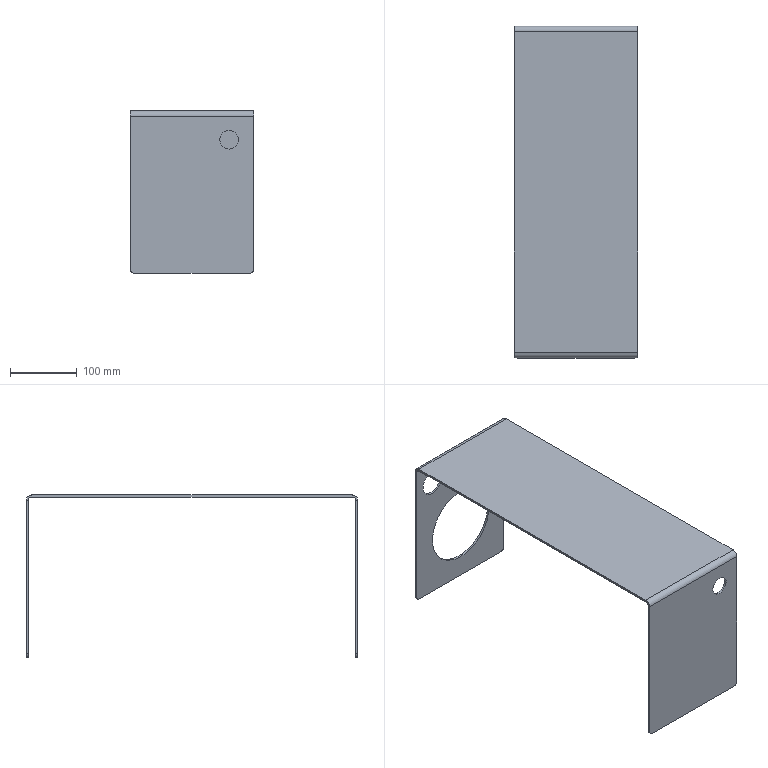Part | SolidWorks | features ICE 2, Fillet 1, FlatPattern 1, SMBaseFlange 1, SheetMetal 1 | 1 solid | 34 faces | box 185 x 497.4 x 243.2 mm | volume 531785 mm3 | plane 18 | cylinder 16 | commonest cylinder face diameters 11 x4 10 x2 16.4 x2 22 x2 28 x2 40 x2
STEP:
#1=CARTESIAN_POINT('',(148.,-494.2,214.));
#2=VERTEX_POINT('',#1);
#3=CARTESIAN_POINT('',(148.,-494.2,186.));
#4=VERTEX_POINT('',#3);
#5=CARTESIAN_POINT('',(148.,-494.2,200.));
#6=DIRECTION('',(0.,-1.,0.));
#7=DIRECTION('',(0.,0.,1.));
#8=AXIS2_PLACEMENT_3D('',#5,#6,#7);
#9=CIRCLE('',#8,14.);
#10=EDGE_CURVE('',#2,#4,#9,.T.);
#11=ORIENTED_EDGE('',*,*,#10,.F.);
#12=CARTESIAN_POINT('',(148.,-497.4,214.));
#13=VERTEX_POINT('',#12);
#14=CARTESIAN_POINT('',(148.,0.001,214.));
#15=DIRECTION('',(0.,-1.,0.));
#16=VECTOR('',#15,1000.);
#17=LINE('',#14,#16);
#18=EDGE_CURVE('',#2,#13,#17,.T.);
#19=ORIENTED_EDGE('',*,*,#18,.T.);
#20=CARTESIAN_POINT('',(148.,-497.4,186.));
#21=VERTEX_POINT('',#20);
#22=CARTESIAN_POINT('',(148.,-497.4,200.));
#23=DIRECTION('',(0.,-1.,0.));
#24=DIRECTION('',(0.,0.,-1.));
#25=AXIS2_PLACEMENT_3D('',#22,#23,#24);
#26=CIRCLE('',#25,14.);
#27=EDGE_CURVE('',#13,#21,#26,.T.);
#28=ORIENTED_EDGE('',*,*,#27,.T.);
#29=CARTESIAN_POINT('',(148.,0.001,186.));
#30=DIRECTION('',(0.,-1.,0.));
#31=VECTOR('',#30,1000.);
#32=LINE('',#29,#31);
#33=EDGE_CURVE('',#4,#21,#32,.T.);
#34=ORIENTED_EDGE('',*,*,#33,.F.);
#35=EDGE_LOOP('',(#11,#19,#28,#34));
#36=FACE_OUTER_BOUND('',#35,.T.);
#37=CARTESIAN_POINT('',(148.,0.001,200.));
#38=DIRECTION('',(0.,-1.,0.));
#39=DIRECTION('',(0.,0.,-1.));
#40=AXIS2_PLACEMENT_3D('',#37,#38,#39);
#41=CYLINDRICAL_SURFACE('',#40,14.);
#42=ADVANCED_FACE('',(#36),#41,.F.);
#43=CARTESIAN_POINT('',(93.5,-3.2,33.5));
#44=VERTEX_POINT('',#43);
#45=CARTESIAN_POINT('',(93.5,-3.2,153.5));
#46=VERTEX_POINT('',#45);
#47=CARTESIAN_POINT('',(93.5,-3.2,93.5));
#48=DIRECTION('',(0.,1.,0.));
#49=DIRECTION('',(0.,0.,-1.));
#50=AXIS2_PLACEMENT_3D('',#47,#48,#49);
#51=CIRCLE('',#50,60.);
#52=EDGE_CURVE('',#44,#46,#51,.T.);
#53=ORIENTED_EDGE('',*,*,#52,.F.);
#54=CARTESIAN_POINT('',(93.5,0.,33.5));
#55=VERTEX_POINT('',#54);
#56=CARTESIAN_POINT('',(93.5,-497.401,33.5));
#57=DIRECTION('',(0.,1.,0.));
#58=VECTOR('',#57,1000.);
#59=LINE('',#56,#58);
#60=EDGE_CURVE('',#44,#55,#59,.T.);
#61=ORIENTED_EDGE('',*,*,#60,.T.);
#62=CARTESIAN_POINT('',(93.5,0.,153.5));
#63=VERTEX_POINT('',#62);
#64=CARTESIAN_POINT('',(93.5,0.,93.5));
#65=DIRECTION('',(0.,1.,0.));
#66=DIRECTION('',(0.,0.,1.));
#67=AXIS2_PLACEMENT_3D('',#64,#65,#66);
#68=CIRCLE('',#67,60.);
#69=EDGE_CURVE('',#55,#63,#68,.T.);
#70=ORIENTED_EDGE('',*,*,#69,.T.);
#71=CARTESIAN_POINT('',(93.5,-497.401,153.5));
#72=DIRECTION('',(0.,1.,0.));
#73=VECTOR('',#72,1000.);
#74=LINE('',#71,#73);
#75=EDGE_CURVE('',#46,#63,#74,.T.);
#76=ORIENTED_EDGE('',*,*,#75,.F.);
#77=EDGE_LOOP('',(#53,#61,#70,#76));
#78=FACE_OUTER_BOUND('',#77,.T.);
#79=CARTESIAN_POINT('',(93.5,-497.401,93.5));
#80=DIRECTION('',(0.,1.,0.));
#81=DIRECTION('',(0.,0.,1.));
#82=AXIS2_PLACEMENT_3D('',#79,#80,#81);
#83=CYLINDRICAL_SURFACE('',#82,60.);
#84=ADVANCED_FACE('',(#78),#83,.F.);
#85=CARTESIAN_POINT('',(105.5,-3.2,195.));
#86=VERTEX_POINT('',#85);
#87=CARTESIAN_POINT('',(105.5,-3.2,217.));
#88=VERTEX_POINT('',#87);
#89=CARTESIAN_POINT('',(105.5,-3.2,206.));
#90=DIRECTION('',(0.,1.,0.));
#91=DIRECTION('',(0.,0.,-1.));
#92=AXIS2_PLACEMENT_3D('',#89,#90,#91);
#93=CIRCLE('',#92,11.);
#94=EDGE_CURVE('',#86,#88,#93,.T.);
#95=ORIENTED_EDGE('',*,*,#94,.F.);
#96=CARTESIAN_POINT('',(105.5,0.,195.));
#97=VERTEX_POINT('',#96);
#98=CARTESIAN_POINT('',(105.5,-497.401,195.));
#99=DIRECTION('',(0.,1.,0.));
#100=VECTOR('',#99,1000.);
#101=LINE('',#98,#100);
#102=EDGE_CURVE('',#86,#97,#101,.T.);
#103=ORIENTED_EDGE('',*,*,#102,.T.);
#104=CARTESIAN_POINT('',(105.5,0.,217.));
#105=VERTEX_POINT('',#104);
#106=CARTESIAN_POINT('',(105.5,0.,206.));
#107=DIRECTION('',(0.,1.,0.));
#108=DIRECTION('',(0.,0.,1.));
#109=AXIS2_PLACEMENT_3D('',#106,#107,#108);
#110=CIRCLE('',#109,11.);
#111=EDGE_CURVE('',#97,#105,#110,.T.);
#112=ORIENTED_EDGE('',*,*,#111,.T.);
#113=CARTESIAN_POINT('',(105.5,-497.401,217.));
#114=DIRECTION('',(0.,1.,0.));
#115=VECTOR('',#114,1000.);
#116=LINE('',#113,#115);
#117=EDGE_CURVE('',#88,#105,#116,.T.);
#118=ORIENTED_EDGE('',*,*,#117,.F.);
#119=EDGE_LOOP('',(#95,#103,#112,#118));
#120=FACE_OUTER_BOUND('',#119,.T.);
#121=CARTESIAN_POINT('',(105.5,-497.401,206.));
#122=DIRECTION('',(0.,1.,0.));
#123=DIRECTION('',(0.,0.,1.));
#124=AXIS2_PLACEMENT_3D('',#121,#122,#123);
#125=CYLINDRICAL_SURFACE('',#124,11.);
#126=ADVANCED_FACE('',(#120),#125,.F.);
#127=CARTESIAN_POINT('',(33.5,-3.2,180.));
#128=VERTEX_POINT('',#127);
#129=CARTESIAN_POINT('',(33.5,-3.2,220.));
#130=VERTEX_POINT('',#129);
#131=CARTESIAN_POINT('',(33.5,-3.2,200.));
#132=DIRECTION('',(0.,1.,0.));
#133=DIRECTION('',(0.,0.,-1.));
#134=AXIS2_PLACEMENT_3D('',#131,#132,#133);
#135=CIRCLE('',#134,20.);
#136=EDGE_CURVE('',#128,#130,#135,.T.);
#137=ORIENTED_EDGE('',*,*,#136,.F.);
#138=CARTESIAN_POINT('',(33.5,0.,180.));
#139=VERTEX_POINT('',#138);
#140=CARTESIAN_POINT('',(33.5,-497.401,180.));
#141=DIRECTION('',(0.,1.,0.));
#142=VECTOR('',#141,1000.);
#143=LINE('',#140,#142);
#144=EDGE_CURVE('',#128,#139,#143,.T.);
#145=ORIENTED_EDGE('',*,*,#144,.T.);
#146=CARTESIAN_POINT('',(33.5,0.,220.));
#147=VERTEX_POINT('',#146);
#148=CARTESIAN_POINT('',(33.5,0.,200.));
#149=DIRECTION('',(0.,1.,0.));
#150=DIRECTION('',(0.,0.,1.));
#151=AXIS2_PLACEMENT_3D('',#148,#149,#150);
#152=CIRCLE('',#151,20.);
#153=EDGE_CURVE('',#139,#147,#152,.T.);
#154=ORIENTED_EDGE('',*,*,#153,.T.);
#155=CARTESIAN_POINT('',(33.5,-497.401,220.));
#156=DIRECTION('',(0.,1.,0.));
#157=VECTOR('',#156,1000.);
#158=LINE('',#155,#157);
#159=EDGE_CURVE('',#130,#147,#158,.T.);
#160=ORIENTED_EDGE('',*,*,#159,.F.);
#161=EDGE_LOOP('',(#137,#145,#154,#160));
#162=FACE_OUTER_BOUND('',#161,.T.);
#163=CARTESIAN_POINT('',(33.5,-497.401,200.));
#164=DIRECTION('',(0.,1.,0.));
#165=DIRECTION('',(0.,0.,1.));
#166=AXIS2_PLACEMENT_3D('',#163,#164,#165);
#167=CYLINDRICAL_SURFACE('',#166,20.);
#168=ADVANCED_FACE('',(#162),#167,.F.);
#169=CARTESIAN_POINT('',(185.,0.,235.));
#170=VERTEX_POINT('',#169);
#171=CARTESIAN_POINT('',(185.,-3.2,235.));
#172=VERTEX_POINT('',#171);
#173=CARTESIAN_POINT('',(185.,0.,235.));
#174=DIRECTION('',(0.,-1.,0.));
#175=VECTOR('',#174,1000.);
#176=LINE('',#173,#175);
#177=EDGE_CURVE('',#170,#172,#176,.T.);
#178=ORIENTED_EDGE('',*,*,#177,.F.);
#179=CARTESIAN_POINT('',(185.,-8.2,243.2));
#180=VERTEX_POINT('',#179);
#181=CARTESIAN_POINT('',(185.,-8.2,235.));
#182=DIRECTION('',(1.,0.,0.));
#183=DIRECTION('',(0.,0.,1.));
#184=AXIS2_PLACEMENT_3D('',#181,#182,#183);
#185=CIRCLE('',#184,8.2);
#186=EDGE_CURVE('',#170,#180,#185,.T.);
#187=ORIENTED_EDGE('',*,*,#186,.T.);
#188=CARTESIAN_POINT('',(185.,-8.2,240.));
#189=VERTEX_POINT('',#188);
#190=CARTESIAN_POINT('',(185.,-8.2,240.));
#191=DIRECTION('',(0.,0.,1.));
#192=VECTOR('',#191,1000.);
#193=LINE('',#190,#192);
#194=EDGE_CURVE('',#189,#180,#193,.T.);
#195=ORIENTED_EDGE('',*,*,#194,.F.);
#196=CARTESIAN_POINT('',(185.,-8.2,235.));
#197=DIRECTION('',(1.,0.,0.));
#198=DIRECTION('',(0.,0.,-1.));
#199=AXIS2_PLACEMENT_3D('',#196,#197,#198);
#200=CIRCLE('',#199,5.);
#201=EDGE_CURVE('',#172,#189,#200,.T.);
#202=ORIENTED_EDGE('',*,*,#201,.F.);
#203=EDGE_LOOP('',(#178,#187,#195,#202));
#204=FACE_OUTER_BOUND('',#203,.T.);
#205=CARTESIAN_POINT('',(185.,0.,235.));
#206=DIRECTION('',(1.,0.,0.));
#207=DIRECTION('',(0.,0.,-1.));
#208=AXIS2_PLACEMENT_3D('',#205,#206,#207);
#209=PLANE('',#208);
#210=ADVANCED_FACE('',(#204),#209,.T.);
#211=CARTESIAN_POINT('',(185.,-3.2,5.5));
#212=VERTEX_POINT('',#211);
#213=CARTESIAN_POINT('',(185.,-3.2,0.));
#214=DIRECTION('',(0.,0.,1.));
#215=VECTOR('',#214,1000.);
#216=LINE('',#213,#215);
#217=EDGE_CURVE('',#212,#172,#216,.T.);
#218=ORIENTED_EDGE('',*,*,#217,.F.);
#219=CARTESIAN_POINT('',(185.,0.,5.5));
#220=VERTEX_POINT('',#219);
#221=CARTESIAN_POINT('',(185.,-8.2,5.5));
#222=DIRECTION('',(0.,1.,0.));
#223=VECTOR('',#222,1000.);
#224=LINE('',#221,#223);
#225=EDGE_CURVE('',#212,#220,#224,.T.);
#226=ORIENTED_EDGE('',*,*,#225,.T.);
#227=CARTESIAN_POINT('',(185.,0.,0.));
#228=DIRECTION('',(0.,0.,1.));
#229=VECTOR('',#228,1000.);
#230=LINE('',#227,#229);
#231=EDGE_CURVE('',#220,#170,#230,.T.);
#232=ORIENTED_EDGE('',*,*,#231,.T.);
#233=ORIENTED_EDGE('',*,*,#177,.T.);
#234=EDGE_LOOP('',(#218,#226,#232,#233));
#235=FACE_OUTER_BOUND('',#234,.T.);
#236=CARTESIAN_POINT('',(185.,-8.2,240.));
#237=DIRECTION('',(1.,0.,0.));
#238=DIRECTION('',(0.,0.,-1.));
#239=AXIS2_PLACEMENT_3D('',#236,#237,#238);
#240=PLANE('',#239);
#241=ADVANCED_FACE('',(#235),#240,.T.);
#242=CARTESIAN_POINT('',(0.,-8.2,243.2));
#243=VERTEX_POINT('',#242);
#244=CARTESIAN_POINT('',(0.,-8.2,240.));
#245=VERTEX_POINT('',#244);
#246=CARTESIAN_POINT('',(0.,-8.2,243.2));
#247=DIRECTION('',(0.,0.,-1.));
#248=VECTOR('',#247,1000.);
#249=LINE('',#246,#248);
#250=EDGE_CURVE('',#243,#245,#249,.T.);
#251=ORIENTED_EDGE('',*,*,#250,.F.);
#252=CARTESIAN_POINT('',(0.,0.,235.));
#253=VERTEX_POINT('',#252);
#254=CARTESIAN_POINT('',(0.,-8.2,235.));
#255=DIRECTION('',(1.,0.,0.));
#256=DIRECTION('',(0.,0.,1.));
#257=AXIS2_PLACEMENT_3D('',#254,#255,#256);
#258=CIRCLE('',#257,8.2);
#259=EDGE_CURVE('',#253,#243,#258,.T.);
#260=ORIENTED_EDGE('',*,*,#259,.F.);
#261=CARTESIAN_POINT('',(0.,-3.2,235.));
#262=VERTEX_POINT('',#261);
#263=CARTESIAN_POINT('',(0.,-3.2,235.));
#264=DIRECTION('',(0.,1.,0.));
#265=VECTOR('',#264,1000.);
#266=LINE('',#263,#265);
#267=EDGE_CURVE('',#262,#253,#266,.T.);
#268=ORIENTED_EDGE('',*,*,#267,.F.);
#269=CARTESIAN_POINT('',(0.,-8.2,235.));
#270=DIRECTION('',(1.,0.,0.));
#271=DIRECTION('',(0.,0.,-1.));
#272=AXIS2_PLACEMENT_3D('',#269,#270,#271);
#273=CIRCLE('',#272,5.);
#274=EDGE_CURVE('',#262,#245,#273,.T.);
#275=ORIENTED_EDGE('',*,*,#274,.T.);
#276=EDGE_LOOP('',(#251,#260,#268,#275));
#277=FACE_OUTER_BOUND('',#276,.T.);
#278=CARTESIAN_POINT('',(0.,-8.2,243.2));
#279=DIRECTION('',(-1.,0.,0.));
#280=DIRECTION('',(0.,0.,1.));
#281=AXIS2_PLACEMENT_3D('',#278,#279,#280);
#282=PLANE('',#281);
#283=ADVANCED_FACE('',(#277),#282,.T.);
#284=CARTESIAN_POINT('',(0.,-489.2,243.2));
#285=VERTEX_POINT('',#284);
#286=CARTESIAN_POINT('',(0.,0.,243.2));
#287=DIRECTION('',(0.,-1.,0.));
#288=VECTOR('',#287,1000.);
#289=LINE('',#286,#288);
#290=EDGE_CURVE('',#243,#285,#289,.T.);
#291=ORIENTED_EDGE('',*,*,#290,.F.);
#292=ORIENTED_EDGE('',*,*,#250,.T.);
#293=CARTESIAN_POINT('',(0.,-489.2,240.));
#294=VERTEX_POINT('',#293);
#295=CARTESIAN_POINT('',(0.,0.,240.));
#296=DIRECTION('',(0.,-1.,0.));
#297=VECTOR('',#296,1000.);
#298=LINE('',#295,#297);
#299=EDGE_CURVE('',#245,#294,#298,.T.);
#300=ORIENTED_EDGE('',*,*,#299,.T.);
#301=CARTESIAN_POINT('',(0.,-489.2,240.));
#302=DIRECTION('',(0.,0.,1.));
#303=VECTOR('',#302,1000.);
#304=LINE('',#301,#303);
#305=EDGE_CURVE('',#294,#285,#304,.T.);
#306=ORIENTED_EDGE('',*,*,#305,.T.);
#307=EDGE_LOOP('',(#291,#292,#300,#306));
#308=FACE_OUTER_BOUND('',#307,.T.);
#309=CARTESIAN_POINT('',(0.,-3.2,235.));
#310=DIRECTION('',(-1.,0.,0.));
#311=DIRECTION('',(0.,0.,1.));
#312=AXIS2_PLACEMENT_3D('',#309,#310,#311);
#313=PLANE('',#312);
#314=ADVANCED_FACE('',(#308),#313,.T.);
#315=CARTESIAN_POINT('',(185.,-489.2,243.2));
#316=VERTEX_POINT('',#315);
#317=CARTESIAN_POINT('',(185.,-489.2,240.));
#318=VERTEX_POINT('',#317);
#319=CARTESIAN_POINT('',(185.,-489.2,243.2));
#320=DIRECTION('',(0.,0.,-1.));
#321=VECTOR('',#320,1000.);
#322=LINE('',#319,#321);
#323=EDGE_CURVE('',#316,#318,#322,.T.);
#324=ORIENTED_EDGE('',*,*,#323,.F.);
#325=CARTESIAN_POINT('',(185.,-497.4,235.));
#326=VERTEX_POINT('',#325);
#327=CARTESIAN_POINT('',(185.,-489.2,235.));
#328=DIRECTION('',(1.,0.,0.));
#329=DIRECTION('',(0.,0.,1.));
#330=AXIS2_PLACEMENT_3D('',#327,#328,#329);
#331=CIRCLE('',#330,8.2);
#332=EDGE_CURVE('',#316,#326,#331,.T.);
#333=ORIENTED_EDGE('',*,*,#332,.T.);
#334=CARTESIAN_POINT('',(185.,-494.2,235.));
#335=VERTEX_POINT('',#334);
#336=CARTESIAN_POINT('',(185.,-494.2,235.));
#337=DIRECTION('',(0.,-1.,0.));
#338=VECTOR('',#337,1000.);
#339=LINE('',#336,#338);
#340=EDGE_CURVE('',#335,#326,#339,.T.);
#341=ORIENTED_EDGE('',*,*,#340,.F.);
#342=CARTESIAN_POINT('',(185.,-489.2,235.));
#343=DIRECTION('',(1.,0.,0.));
#344=DIRECTION('',(0.,0.,-1.));
#345=AXIS2_PLACEMENT_3D('',#342,#343,#344);
#346=CIRCLE('',#345,5.);
#347=EDGE_CURVE('',#318,#335,#346,.T.);
#348=ORIENTED_EDGE('',*,*,#347,.F.);
#349=EDGE_LOOP('',(#324,#333,#341,#348));
#350=FACE_OUTER_BOUND('',#349,.T.);
#351=CARTESIAN_POINT('',(185.,-489.2,243.2));
#352=DIRECTION('',(1.,0.,0.));
#353=DIRECTION('',(0.,0.,-1.));
#354=AXIS2_PLACEMENT_3D('',#351,#352,#353);
#355=PLANE('',#354);
#356=ADVANCED_FACE('',(#350),#355,.T.);
#357=CARTESIAN_POINT('',(185.,0.,243.2));
#358=DIRECTION('',(0.,-1.,0.));
#359=VECTOR('',#358,1000.);
#360=LINE('',#357,#359);
#361=EDGE_CURVE('',#180,#316,#360,.T.);
#362=ORIENTED_EDGE('',*,*,#361,.T.);
#363=ORIENTED_EDGE('',*,*,#323,.T.);
#364=CARTESIAN_POINT('',(185.,0.,240.));
#365=DIRECTION('',(0.,-1.,0.));
#366=VECTOR('',#365,1000.);
#367=LINE('',#364,#366);
#368=EDGE_CURVE('',#189,#318,#367,.T.);
#369=ORIENTED_EDGE('',*,*,#368,.F.);
#370=ORIENTED_EDGE('',*,*,#194,.T.);
#371=EDGE_LOOP('',(#362,#363,#369,#370));
#372=FACE_OUTER_BOUND('',#371,.T.);
#373=CARTESIAN_POINT('',(185.,-494.2,235.));
#374=DIRECTION('',(1.,0.,0.));
#375=DIRECTION('',(0.,0.,-1.));
#376=AXIS2_PLACEMENT_3D('',#373,#374,#375);
#377=PLANE('',#376);
#378=ADVANCED_FACE('',(#372),#377,.T.);
#379=CARTESIAN_POINT('',(0.,-497.4,235.));
#380=VERTEX_POINT('',#379);
#381=CARTESIAN_POINT('',(0.,-494.2,235.));
#382=VERTEX_POINT('',#381);
#383=CARTESIAN_POINT('',(0.,-497.4,235.));
#384=DIRECTION('',(0.,1.,0.));
#385=VECTOR('',#384,1000.);
#386=LINE('',#383,#385);
#387=EDGE_CURVE('',#380,#382,#386,.T.);
#388=ORIENTED_EDGE('',*,*,#387,.F.);
#389=CARTESIAN_POINT('',(0.,-489.2,235.));
#390=DIRECTION('',(1.,0.,0.));
#391=DIRECTION('',(0.,0.,1.));
#392=AXIS2_PLACEMENT_3D('',#389,#390,#391);
#393=CIRCLE('',#392,8.2);
#394=EDGE_CURVE('',#285,#380,#393,.T.);
#395=ORIENTED_EDGE('',*,*,#394,.F.);
#396=ORIENTED_EDGE('',*,*,#305,.F.);
#397=CARTESIAN_POINT('',(0.,-489.2,235.));
#398=DIRECTION('',(1.,0.,0.));
#399=DIRECTION('',(0.,0.,-1.));
#400=AXIS2_PLACEMENT_3D('',#397,#398,#399);
#401=CIRCLE('',#400,5.);
#402=EDGE_CURVE('',#294,#382,#401,.T.);
#403=ORIENTED_EDGE('',*,*,#402,.T.);
#404=EDGE_LOOP('',(#388,#395,#396,#403));
#405=FACE_OUTER_BOUND('',#404,.T.);
#406=CARTESIAN_POINT('',(0.,-497.4,235.));
#407=DIRECTION('',(-1.,0.,0.));
#408=DIRECTION('',(0.,0.,1.));
#409=AXIS2_PLACEMENT_3D('',#406,#407,#408);
#410=PLANE('',#409);
#411=ADVANCED_FACE('',(#405),#410,.T.);
#412=CARTESIAN_POINT('',(0.,-494.2,5.5));
#413=VERTEX_POINT('',#412);
#414=CARTESIAN_POINT('',(0.,-494.2,243.2));
#415=DIRECTION('',(0.,0.,-1.));
#416=VECTOR('',#415,1000.);
#417=LINE('',#414,#416);
#418=EDGE_CURVE('',#382,#413,#417,.T.);
#419=ORIENTED_EDGE('',*,*,#418,.T.);
#420=CARTESIAN_POINT('',(0.,-497.4,5.5));
#421=VERTEX_POINT('',#420);
#422=CARTESIAN_POINT('',(0.,-489.2,5.5));
#423=DIRECTION('',(0.,-1.,0.));
#424=VECTOR('',#423,1000.);
#425=LINE('',#422,#424);
#426=EDGE_CURVE('',#413,#421,#425,.T.);
#427=ORIENTED_EDGE('',*,*,#426,.T.);
#428=CARTESIAN_POINT('',(0.,-497.4,243.2));
#429=DIRECTION('',(0.,0.,-1.));
#430=VECTOR('',#429,1000.);
#431=LINE('',#428,#430);
#432=EDGE_CURVE('',#380,#421,#431,.T.);
#433=ORIENTED_EDGE('',*,*,#432,.F.);
#434=ORIENTED_EDGE('',*,*,#387,.T.);
#435=EDGE_LOOP('',(#419,#427,#433,#434));
#436=FACE_OUTER_BOUND('',#435,.T.);
#437=CARTESIAN_POINT('',(0.,-489.2,240.));
#438=DIRECTION('',(-1.,0.,0.));
#439=DIRECTION('',(0.,0.,1.));
#440=AXIS2_PLACEMENT_3D('',#437,#438,#439);
#441=PLANE('',#440);
#442=ADVANCED_FACE('',(#436),#441,.T.);
#443=CARTESIAN_POINT('',(148.,-497.4,200.));
#444=DIRECTION('',(0.,-1.,0.));
#445=DIRECTION('',(0.,0.,-1.));
#446=AXIS2_PLACEMENT_3D('',#443,#444,#445);
#447=CIRCLE('',#446,14.);
#448=EDGE_CURVE('',#21,#13,#447,.T.);
#449=ORIENTED_EDGE('',*,*,#448,.F.);
#450=ORIENTED_EDGE('',*,*,#27,.F.);
#451=EDGE_LOOP('',(#449,#450));
#452=FACE_BOUND('',#451,.T.);
#453=CARTESIAN_POINT('',(179.5,-497.4,0.));
#454=VERTEX_POINT('',#453);
#455=CARTESIAN_POINT('',(5.5,-497.4,0.));
#456=VERTEX_POINT('',#455);
#457=CARTESIAN_POINT('',(185.,-497.4,0.));
#458=DIRECTION('',(-1.,0.,0.));
#459=VECTOR('',#458,1000.);
#460=LINE('',#457,#459);
#461=EDGE_CURVE('',#454,#456,#460,.T.);
#462=ORIENTED_EDGE('',*,*,#461,.F.);
#463=CARTESIAN_POINT('',(185.,-497.4,5.5));
#464=VERTEX_POINT('',#463);
#465=CARTESIAN_POINT('',(179.5,-497.4,5.5));
#466=DIRECTION('',(0.,-1.,0.));
#467=DIRECTION('',(0.,0.,1.));
#468=AXIS2_PLACEMENT_3D('',#465,#466,#467);
#469=CIRCLE('',#468,5.5);
#470=EDGE_CURVE('',#454,#464,#469,.T.);
#471=ORIENTED_EDGE('',*,*,#470,.T.);
#472=CARTESIAN_POINT('',(185.,-497.4,243.2));
#473=DIRECTION('',(0.,0.,-1.));
#474=VECTOR('',#473,1000.);
#475=LINE('',#472,#474);
#476=EDGE_CURVE('',#326,#464,#475,.T.);
#477=ORIENTED_EDGE('',*,*,#476,.F.);
#478=CARTESIAN_POINT('',(185.,-497.4,235.));
#479=DIRECTION('',(-1.,0.,0.));
#480=VECTOR('',#479,1000.);
#481=LINE('',#478,#480);
#482=EDGE_CURVE('',#326,#380,#481,.T.);
#483=ORIENTED_EDGE('',*,*,#482,.T.);
#484=ORIENTED_EDGE('',*,*,#432,.T.);
#485=CARTESIAN_POINT('',(5.5,-497.4,5.5));
#486=DIRECTION('',(0.,-1.,0.));
#487=DIRECTION('',(0.,0.,1.));
#488=AXIS2_PLACEMENT_3D('',#485,#486,#487);
#489=CIRCLE('',#488,5.5);
#490=EDGE_CURVE('',#421,#456,#489,.T.);
#491=ORIENTED_EDGE('',*,*,#490,.T.);
#492=EDGE_LOOP('',(#462,#471,#477,#483,#484,#491));
#493=FACE_OUTER_BOUND('',#492,.T.);
#494=CARTESIAN_POINT('',(185.,-497.4,243.2));
#495=DIRECTION('',(0.,1.,0.));
#496=DIRECTION('',(0.,0.,1.));
#497=AXIS2_PLACEMENT_3D('',#494,#495,#496);
#498=PLANE('',#497);
#499=ADVANCED_FACE('',(#452,#493),#498,.F.);
#500=CARTESIAN_POINT('',(179.5,-494.2,0.));
#501=VERTEX_POINT('',#500);
#502=CARTESIAN_POINT('',(5.5,-494.2,0.));
#503=VERTEX_POINT('',#502);
#504=CARTESIAN_POINT('',(185.,-494.2,0.));
#505=DIRECTION('',(-1.,0.,0.));
#506=VECTOR('',#505,1000.);
#507=LINE('',#504,#506);
#508=EDGE_CURVE('',#501,#503,#507,.T.);
#509=ORIENTED_EDGE('',*,*,#508,.F.);
#510=CARTESIAN_POINT('',(179.5,-494.2,0.));
#511=DIRECTION('',(0.,-1.,0.));
#512=VECTOR('',#511,1000.);
#513=LINE('',#510,#512);
#514=EDGE_CURVE('',#501,#454,#513,.T.);
#515=ORIENTED_EDGE('',*,*,#514,.T.);
#516=ORIENTED_EDGE('',*,*,#461,.T.);
#517=CARTESIAN_POINT('',(5.5,-494.2,0.));
#518=DIRECTION('',(0.,1.,0.));
#519=VECTOR('',#518,1000.);
#520=LINE('',#517,#519);
#521=EDGE_CURVE('',#456,#503,#520,.T.);
#522=ORIENTED_EDGE('',*,*,#521,.T.);
#523=EDGE_LOOP('',(#509,#515,#516,#522));
#524=FACE_OUTER_BOUND('',#523,.T.);
#525=CARTESIAN_POINT('',(185.,-494.2,0.));
#526=DIRECTION('',(0.,0.,-1.));
#527=DIRECTION('',(-1.,0.,0.));
#528=AXIS2_PLACEMENT_3D('',#525,#526,#527);
#529=PLANE('',#528);
#530=ADVANCED_FACE('',(#524),#529,.T.);
#531=CARTESIAN_POINT('',(148.,-494.2,200.));
#532=DIRECTION('',(0.,-1.,0.));
#533=DIRECTION('',(0.,0.,1.));
#534=AXIS2_PLACEMENT_3D('',#531,#532,#533);
#535=CIRCLE('',#534,14.);
#536=EDGE_CURVE('',#4,#2,#535,.T.);
#537=ORIENTED_EDGE('',*,*,#536,.T.);
#538=ORIENTED_EDGE('',*,*,#10,.T.);
#539=EDGE_LOOP('',(#537,#538));
#540=FACE_BOUND('',#539,.T.);
#541=CARTESIAN_POINT('',(185.,-494.2,5.5));
#542=VERTEX_POINT('',#541);
#543=CARTESIAN_POINT('',(185.,-494.2,243.2));
#544=DIRECTION('',(0.,0.,-1.));
#545=VECTOR('',#544,1000.);
#546=LINE('',#543,#545);
#547=EDGE_CURVE('',#335,#542,#546,.T.);
#548=ORIENTED_EDGE('',*,*,#547,.T.);
#549=CARTESIAN_POINT('',(179.5,-494.2,5.5));
#550=DIRECTION('',(0.,1.,0.));
#551=DIRECTION('',(0.,0.,1.));
#552=AXIS2_PLACEMENT_3D('',#549,#550,#551);
#553=CIRCLE('',#552,5.5);
#554=EDGE_CURVE('',#542,#501,#553,.T.);
#555=ORIENTED_EDGE('',*,*,#554,.T.);
#556=ORIENTED_EDGE('',*,*,#508,.T.);
#557=CARTESIAN_POINT('',(5.5,-494.2,5.5));
#558=DIRECTION('',(0.,1.,0.));
#559=DIRECTION('',(0.,0.,1.));
#560=AXIS2_PLACEMENT_3D('',#557,#558,#559);
#561=CIRCLE('',#560,5.5);
#562=EDGE_CURVE('',#503,#413,#561,.T.);
#563=ORIENTED_EDGE('',*,*,#562,.T.);
#564=ORIENTED_EDGE('',*,*,#418,.F.);
#565=CARTESIAN_POINT('',(185.,-494.2,235.));
#566=DIRECTION('',(-1.,0.,0.));
#567=VECTOR('',#566,1000.);
#568=LINE('',#565,#567);
#569=EDGE_CURVE('',#335,#382,#568,.T.);
#570=ORIENTED_EDGE('',*,*,#569,.F.);
#571=EDGE_LOOP('',(#548,#555,#556,#563,#564,#570));
#572=FACE_OUTER_BOUND('',#571,.T.);
#573=CARTESIAN_POINT('',(185.,-494.2,243.2));
#574=DIRECTION('',(0.,1.,0.));
#575=DIRECTION('',(0.,0.,1.));
#576=AXIS2_PLACEMENT_3D('',#573,#574,#575);
#577=PLANE('',#576);
#578=ADVANCED_FACE('',(#540,#572),#577,.T.);
#579=ORIENTED_EDGE('',*,*,#402,.F.);
#580=CARTESIAN_POINT('',(185.,-489.2,240.));
#581=DIRECTION('',(-1.,0.,0.));
#582=VECTOR('',#581,1000.);
#583=LINE('',#580,#582);
#584=EDGE_CURVE('',#318,#294,#583,.T.);
#585=ORIENTED_EDGE('',*,*,#584,.F.);
#586=ORIENTED_EDGE('',*,*,#347,.T.);
#587=ORIENTED_EDGE('',*,*,#569,.T.);
#588=EDGE_LOOP('',(#579,#585,#586,#587));
#589=FACE_OUTER_BOUND('',#588,.T.);
#590=CARTESIAN_POINT('',(185.,-489.2,235.));
#591=DIRECTION('',(-1.,0.,0.));
#592=DIRECTION('',(0.,0.,1.));
#593=AXIS2_PLACEMENT_3D('',#590,#591,#592);
#594=CYLINDRICAL_SURFACE('',#593,5.);
#595=ADVANCED_FACE('',(#589),#594,.F.);
#596=ORIENTED_EDGE('',*,*,#299,.F.);
#597=CARTESIAN_POINT('',(185.,-8.2,240.));
#598=DIRECTION('',(-1.,0.,0.));
#599=VECTOR('',#598,1000.);
#600=LINE('',#597,#599);
#601=EDGE_CURVE('',#189,#245,#600,.T.);
#602=ORIENTED_EDGE('',*,*,#601,.F.);
#603=ORIENTED_EDGE('',*,*,#368,.T.);
#604=ORIENTED_EDGE('',*,*,#584,.T.);
#605=EDGE_LOOP('',(#596,#602,#603,#604));
#606=FACE_OUTER_BOUND('',#605,.T.);
#607=CARTESIAN_POINT('',(185.,0.,240.));
#608=DIRECTION('',(0.,0.,-1.));
#609=DIRECTION('',(0.,1.,0.));
#610=AXIS2_PLACEMENT_3D('',#607,#608,#609);
#611=PLANE('',#610);
#612=ADVANCED_FACE('',(#606),#611,.T.);
#613=ORIENTED_EDGE('',*,*,#274,.F.);
#614=CARTESIAN_POINT('',(185.,-3.2,235.));
#615=DIRECTION('',(-1.,0.,0.));
#616=VECTOR('',#615,1000.);
#617=LINE('',#614,#616);
#618=EDGE_CURVE('',#172,#262,#617,.T.);
#619=ORIENTED_EDGE('',*,*,#618,.F.);
#620=ORIENTED_EDGE('',*,*,#201,.T.);
#621=ORIENTED_EDGE('',*,*,#601,.T.);
#622=EDGE_LOOP('',(#613,#619,#620,#621));
#623=FACE_OUTER_BOUND('',#622,.T.);
#624=CARTESIAN_POINT('',(185.,-8.2,235.));
#625=DIRECTION('',(-1.,0.,0.));
#626=DIRECTION('',(0.,0.,1.));
#627=AXIS2_PLACEMENT_3D('',#624,#625,#626);
#628=CYLINDRICAL_SURFACE('',#627,5.);
#629=ADVANCED_FACE('',(#623),#628,.F.);
#630=CARTESIAN_POINT('',(93.5,-3.2,93.5));
#631=DIRECTION('',(0.,1.,0.));
#632=DIRECTION('',(0.,0.,-1.));
#633=AXIS2_PLACEMENT_3D('',#630,#631,#632);
#634=CIRCLE('',#633,60.);
#635=EDGE_CURVE('',#46,#44,#634,.T.);
#636=ORIENTED_EDGE('',*,*,#635,.T.);
#637=ORIENTED_EDGE('',*,*,#52,.T.);
#638=EDGE_LOOP('',(#636,#637));
#639=FACE_BOUND('',#638,.T.);
#640=CARTESIAN_POINT('',(105.5,-3.2,206.));
#641=DIRECTION('',(0.,1.,0.));
#642=DIRECTION('',(0.,0.,-1.));
#643=AXIS2_PLACEMENT_3D('',#640,#641,#642);
#644=CIRCLE('',#643,11.);
#645=EDGE_CURVE('',#88,#86,#644,.T.);
#646=ORIENTED_EDGE('',*,*,#645,.T.);
#647=ORIENTED_EDGE('',*,*,#94,.T.);
#648=EDGE_LOOP('',(#646,#647));
#649=FACE_BOUND('',#648,.T.);
#650=CARTESIAN_POINT('',(33.5,-3.2,200.));
#651=DIRECTION('',(0.,1.,0.));
#652=DIRECTION('',(0.,0.,-1.));
#653=AXIS2_PLACEMENT_3D('',#650,#651,#652);
#654=CIRCLE('',#653,20.);
#655=EDGE_CURVE('',#130,#128,#654,.T.);
#656=ORIENTED_EDGE('',*,*,#655,.T.);
#657=ORIENTED_EDGE('',*,*,#136,.T.);
#658=EDGE_LOOP('',(#656,#657));
#659=FACE_BOUND('',#658,.T.);
#660=CARTESIAN_POINT('',(0.,-3.2,5.5));
#661=VERTEX_POINT('',#660);
#662=CARTESIAN_POINT('',(0.,-3.2,0.));
#663=DIRECTION('',(0.,0.,1.));
#664=VECTOR('',#663,1000.);
#665=LINE('',#662,#664);
#666=EDGE_CURVE('',#661,#262,#665,.T.);
#667=ORIENTED_EDGE('',*,*,#666,.F.);
#668=CARTESIAN_POINT('',(5.5,-3.2,0.));
#669=VERTEX_POINT('',#668);
#670=CARTESIAN_POINT('',(5.5,-3.2,5.5));
#671=DIRECTION('',(0.,-1.,0.));
#672=DIRECTION('',(0.,0.,-1.));
#673=AXIS2_PLACEMENT_3D('',#670,#671,#672);
#674=CIRCLE('',#673,5.5);
#675=EDGE_CURVE('',#661,#669,#674,.T.);
#676=ORIENTED_EDGE('',*,*,#675,.T.);
#677=CARTESIAN_POINT('',(179.5,-3.2,0.));
#678=VERTEX_POINT('',#677);
#679=CARTESIAN_POINT('',(185.,-3.2,0.));
#680=DIRECTION('',(-1.,0.,0.));
#681=VECTOR('',#680,1000.);
#682=LINE('',#679,#681);
#683=EDGE_CURVE('',#678,#669,#682,.T.);
#684=ORIENTED_EDGE('',*,*,#683,.F.);
#685=CARTESIAN_POINT('',(179.5,-3.2,5.5));
#686=DIRECTION('',(0.,-1.,0.));
#687=DIRECTION('',(0.,0.,-1.));
#688=AXIS2_PLACEMENT_3D('',#685,#686,#687);
#689=CIRCLE('',#688,5.5);
#690=EDGE_CURVE('',#678,#212,#689,.T.);
#691=ORIENTED_EDGE('',*,*,#690,.T.);
#692=ORIENTED_EDGE('',*,*,#217,.T.);
#693=ORIENTED_EDGE('',*,*,#618,.T.);
#694=EDGE_LOOP('',(#667,#676,#684,#691,#692,#693));
#695=FACE_OUTER_BOUND('',#694,.T.);
#696=CARTESIAN_POINT('',(185.,-3.2,0.));
#697=DIRECTION('',(0.,-1.,0.));
#698=DIRECTION('',(0.,0.,-1.));
#699=AXIS2_PLACEMENT_3D('',#696,#697,#698);
#700=PLANE('',#699);
#701=ADVANCED_FACE('',(#639,#649,#659,#695),#700,.T.);
#702=ORIENTED_EDGE('',*,*,#683,.T.);
#703=CARTESIAN_POINT('',(5.5,0.,0.));
#704=VERTEX_POINT('',#703);
#705=CARTESIAN_POINT('',(5.5,0.,0.));
#706=DIRECTION('',(0.,1.,0.));
#707=VECTOR('',#706,1000.);
#708=LINE('',#705,#707);
#709=EDGE_CURVE('',#669,#704,#708,.T.);
#710=ORIENTED_EDGE('',*,*,#709,.T.);
#711=CARTESIAN_POINT('',(179.5,0.,0.));
#712=VERTEX_POINT('',#711);
#713=CARTESIAN_POINT('',(185.,0.,0.));
#714=DIRECTION('',(-1.,0.,0.));
#715=VECTOR('',#714,1000.);
#716=LINE('',#713,#715);
#717=EDGE_CURVE('',#712,#704,#716,.T.);
#718=ORIENTED_EDGE('',*,*,#717,.F.);
#719=CARTESIAN_POINT('',(179.5,0.,0.));
#720=DIRECTION('',(0.,-1.,0.));
#721=VECTOR('',#720,1000.);
#722=LINE('',#719,#721);
#723=EDGE_CURVE('',#712,#678,#722,.T.);
#724=ORIENTED_EDGE('',*,*,#723,.T.);
#725=EDGE_LOOP('',(#702,#710,#718,#724));
#726=FACE_OUTER_BOUND('',#725,.T.);
#727=CARTESIAN_POINT('',(185.,0.,0.));
#728=DIRECTION('',(0.,0.,-1.));
#729=DIRECTION('',(0.,1.,0.));
#730=AXIS2_PLACEMENT_3D('',#727,#728,#729);
#731=PLANE('',#730);
#732=ADVANCED_FACE('',(#726),#731,.T.);
#733=CARTESIAN_POINT('',(93.5,0.,93.5));
#734=DIRECTION('',(0.,1.,0.));
#735=DIRECTION('',(0.,0.,1.));
#736=AXIS2_PLACEMENT_3D('',#733,#734,#735);
#737=CIRCLE('',#736,60.);
#738=EDGE_CURVE('',#63,#55,#737,.T.);
#739=ORIENTED_EDGE('',*,*,#738,.F.);
#740=ORIENTED_EDGE('',*,*,#69,.F.);
#741=EDGE_LOOP('',(#739,#740));
#742=FACE_BOUND('',#741,.T.);
#743=CARTESIAN_POINT('',(105.5,0.,206.));
#744=DIRECTION('',(0.,1.,0.));
#745=DIRECTION('',(0.,0.,1.));
#746=AXIS2_PLACEMENT_3D('',#743,#744,#745);
#747=CIRCLE('',#746,11.);
#748=EDGE_CURVE('',#105,#97,#747,.T.);
#749=ORIENTED_EDGE('',*,*,#748,.F.);
#750=ORIENTED_EDGE('',*,*,#111,.F.);
#751=EDGE_LOOP('',(#749,#750));
#752=FACE_BOUND('',#751,.T.);
#753=CARTESIAN_POINT('',(33.5,0.,200.));
#754=DIRECTION('',(0.,1.,0.));
#755=DIRECTION('',(0.,0.,1.));
#756=AXIS2_PLACEMENT_3D('',#753,#754,#755);
#757=CIRCLE('',#756,20.);
#758=EDGE_CURVE('',#147,#139,#757,.T.);
#759=ORIENTED_EDGE('',*,*,#758,.F.);
#760=ORIENTED_EDGE('',*,*,#153,.F.);
#761=EDGE_LOOP('',(#759,#760));
#762=FACE_BOUND('',#761,.T.);
#763=ORIENTED_EDGE('',*,*,#717,.T.);
#764=CARTESIAN_POINT('',(0.,0.,5.5));
#765=VERTEX_POINT('',#764);
#766=CARTESIAN_POINT('',(5.5,0.,5.5));
#767=DIRECTION('',(0.,1.,0.));
#768=DIRECTION('',(0.,0.,-1.));
#769=AXIS2_PLACEMENT_3D('',#766,#767,#768);
#770=CIRCLE('',#769,5.5);
#771=EDGE_CURVE('',#704,#765,#770,.T.);
#772=ORIENTED_EDGE('',*,*,#771,.T.);
#773=CARTESIAN_POINT('',(0.,0.,0.));
#774=DIRECTION('',(0.,0.,1.));
#775=VECTOR('',#774,1000.);
#776=LINE('',#773,#775);
#777=EDGE_CURVE('',#765,#253,#776,.T.);
#778=ORIENTED_EDGE('',*,*,#777,.T.);
#779=CARTESIAN_POINT('',(185.,0.,235.));
#780=DIRECTION('',(-1.,0.,0.));
#781=VECTOR('',#780,1000.);
#782=LINE('',#779,#781);
#783=EDGE_CURVE('',#170,#253,#782,.T.);
#784=ORIENTED_EDGE('',*,*,#783,.F.);
#785=ORIENTED_EDGE('',*,*,#231,.F.);
#786=CARTESIAN_POINT('',(179.5,0.,5.5));
#787=DIRECTION('',(0.,1.,0.));
#788=DIRECTION('',(0.,0.,-1.));
#789=AXIS2_PLACEMENT_3D('',#786,#787,#788);
#790=CIRCLE('',#789,5.5);
#791=EDGE_CURVE('',#220,#712,#790,.T.);
#792=ORIENTED_EDGE('',*,*,#791,.T.);
#793=EDGE_LOOP('',(#763,#772,#778,#784,#785,#792));
#794=FACE_OUTER_BOUND('',#793,.T.);
#795=CARTESIAN_POINT('',(185.,0.,0.));
#796=DIRECTION('',(0.,-1.,0.));
#797=DIRECTION('',(0.,0.,-1.));
#798=AXIS2_PLACEMENT_3D('',#795,#796,#797);
#799=PLANE('',#798);
#800=ADVANCED_FACE('',(#742,#752,#762,#794),#799,.F.);
#801=ORIENTED_EDGE('',*,*,#259,.T.);
#802=CARTESIAN_POINT('',(185.,-8.2,243.2));
#803=DIRECTION('',(-1.,0.,0.));
#804=VECTOR('',#803,1000.);
#805=LINE('',#802,#804);
#806=EDGE_CURVE('',#180,#243,#805,.T.);
#807=ORIENTED_EDGE('',*,*,#806,.F.);
#808=ORIENTED_EDGE('',*,*,#186,.F.);
#809=ORIENTED_EDGE('',*,*,#783,.T.);
#810=EDGE_LOOP('',(#801,#807,#808,#809));
#811=FACE_OUTER_BOUND('',#810,.T.);
#812=CARTESIAN_POINT('',(185.,-8.2,235.));
#813=DIRECTION('',(-1.,0.,0.));
#814=DIRECTION('',(0.,0.,1.));
#815=AXIS2_PLACEMENT_3D('',#812,#813,#814);
#816=CYLINDRICAL_SURFACE('',#815,8.2);
#817=ADVANCED_FACE('',(#811),#816,.T.);
#818=ORIENTED_EDGE('',*,*,#290,.T.);
#819=CARTESIAN_POINT('',(185.,-489.2,243.2));
#820=DIRECTION('',(-1.,0.,0.));
#821=VECTOR('',#820,1000.);
#822=LINE('',#819,#821);
#823=EDGE_CURVE('',#316,#285,#822,.T.);
#824=ORIENTED_EDGE('',*,*,#823,.F.);
#825=ORIENTED_EDGE('',*,*,#361,.F.);
#826=ORIENTED_EDGE('',*,*,#806,.T.);
#827=EDGE_LOOP('',(#818,#824,#825,#826));
#828=FACE_OUTER_BOUND('',#827,.T.);
#829=CARTESIAN_POINT('',(185.,0.,243.2));
#830=DIRECTION('',(0.,0.,-1.));
#831=DIRECTION('',(0.,1.,0.));
#832=AXIS2_PLACEMENT_3D('',#829,#830,#831);
#833=PLANE('',#832);
#834=ADVANCED_FACE('',(#828),#833,.F.);
#835=ORIENTED_EDGE('',*,*,#394,.T.);
#836=ORIENTED_EDGE('',*,*,#482,.F.);
#837=ORIENTED_EDGE('',*,*,#332,.F.);
#838=ORIENTED_EDGE('',*,*,#823,.T.);
#839=EDGE_LOOP('',(#835,#836,#837,#838));
#840=FACE_OUTER_BOUND('',#839,.T.);
#841=CARTESIAN_POINT('',(185.,-489.2,235.));
#842=DIRECTION('',(-1.,0.,0.));
#843=DIRECTION('',(0.,0.,1.));
#844=AXIS2_PLACEMENT_3D('',#841,#842,#843);
#845=CYLINDRICAL_SURFACE('',#844,8.2);
#846=ADVANCED_FACE('',(#840),#845,.T.);
#847=ORIENTED_EDGE('',*,*,#476,.T.);
#848=CARTESIAN_POINT('',(185.,-489.2,5.5));
#849=DIRECTION('',(0.,1.,0.));
#850=VECTOR('',#849,1000.);
#851=LINE('',#848,#850);
#852=EDGE_CURVE('',#464,#542,#851,.T.);
#853=ORIENTED_EDGE('',*,*,#852,.T.);
#854=ORIENTED_EDGE('',*,*,#547,.F.);
#855=ORIENTED_EDGE('',*,*,#340,.T.);
#856=EDGE_LOOP('',(#847,#853,#854,#855));
#857=FACE_OUTER_BOUND('',#856,.T.);
#858=CARTESIAN_POINT('',(185.,-489.2,235.));
#859=DIRECTION('',(1.,0.,0.));
#860=DIRECTION('',(0.,0.,-1.));
#861=AXIS2_PLACEMENT_3D('',#858,#859,#860);
#862=PLANE('',#861);
#863=ADVANCED_FACE('',(#857),#862,.T.);
#864=ORIENTED_EDGE('',*,*,#777,.F.);
#865=CARTESIAN_POINT('',(0.,-3.2,5.5));
#866=DIRECTION('',(0.,-1.,0.));
#867=VECTOR('',#866,1000.);
#868=LINE('',#865,#867);
#869=EDGE_CURVE('',#765,#661,#868,.T.);
#870=ORIENTED_EDGE('',*,*,#869,.T.);
#871=ORIENTED_EDGE('',*,*,#666,.T.);
#872=ORIENTED_EDGE('',*,*,#267,.T.);
#873=EDGE_LOOP('',(#864,#870,#871,#872));
#874=FACE_OUTER_BOUND('',#873,.T.);
#875=CARTESIAN_POINT('',(0.,-489.2,235.));
#876=DIRECTION('',(1.,0.,0.));
#877=DIRECTION('',(0.,0.,-1.));
#878=AXIS2_PLACEMENT_3D('',#875,#876,#877);
#879=PLANE('',#878);
#880=ADVANCED_FACE('',(#874),#879,.F.);
#881=ORIENTED_EDGE('',*,*,#144,.F.);
#882=ORIENTED_EDGE('',*,*,#655,.F.);
#883=ORIENTED_EDGE('',*,*,#159,.T.);
#884=ORIENTED_EDGE('',*,*,#758,.T.);
#885=EDGE_LOOP('',(#881,#882,#883,#884));
#886=FACE_OUTER_BOUND('',#885,.T.);
#887=CARTESIAN_POINT('',(33.5,-497.401,200.));
#888=DIRECTION('',(0.,1.,0.));
#889=DIRECTION('',(0.,0.,1.));
#890=AXIS2_PLACEMENT_3D('',#887,#888,#889);
#891=CYLINDRICAL_SURFACE('',#890,20.);
#892=ADVANCED_FACE('',(#886),#891,.F.);
#893=ORIENTED_EDGE('',*,*,#102,.F.);
#894=ORIENTED_EDGE('',*,*,#645,.F.);
#895=ORIENTED_EDGE('',*,*,#117,.T.);
#896=ORIENTED_EDGE('',*,*,#748,.T.);
#897=EDGE_LOOP('',(#893,#894,#895,#896));
#898=FACE_OUTER_BOUND('',#897,.T.);
#899=CARTESIAN_POINT('',(105.5,-497.401,206.));
#900=DIRECTION('',(0.,1.,0.));
#901=DIRECTION('',(0.,0.,1.));
#902=AXIS2_PLACEMENT_3D('',#899,#900,#901);
#903=CYLINDRICAL_SURFACE('',#902,11.);
#904=ADVANCED_FACE('',(#898),#903,.F.);
#905=ORIENTED_EDGE('',*,*,#60,.F.);
#906=ORIENTED_EDGE('',*,*,#635,.F.);
#907=ORIENTED_EDGE('',*,*,#75,.T.);
#908=ORIENTED_EDGE('',*,*,#738,.T.);
#909=EDGE_LOOP('',(#905,#906,#907,#908));
#910=FACE_OUTER_BOUND('',#909,.T.);
#911=CARTESIAN_POINT('',(93.5,-497.401,93.5));
#912=DIRECTION('',(0.,1.,0.));
#913=DIRECTION('',(0.,0.,1.));
#914=AXIS2_PLACEMENT_3D('',#911,#912,#913);
#915=CYLINDRICAL_SURFACE('',#914,60.);
#916=ADVANCED_FACE('',(#910),#915,.F.);
#917=ORIENTED_EDGE('',*,*,#18,.F.);
#918=ORIENTED_EDGE('',*,*,#536,.F.);
#919=ORIENTED_EDGE('',*,*,#33,.T.);
#920=ORIENTED_EDGE('',*,*,#448,.T.);
#921=EDGE_LOOP('',(#917,#918,#919,#920));
#922=FACE_OUTER_BOUND('',#921,.T.);
#923=CARTESIAN_POINT('',(148.,0.001,200.));
#924=DIRECTION('',(0.,-1.,0.));
#925=DIRECTION('',(0.,0.,-1.));
#926=AXIS2_PLACEMENT_3D('',#923,#924,#925);
#927=CYLINDRICAL_SURFACE('',#926,14.);
#928=ADVANCED_FACE('',(#922),#927,.F.);
#929=ORIENTED_EDGE('',*,*,#554,.F.);
#930=ORIENTED_EDGE('',*,*,#852,.F.);
#931=ORIENTED_EDGE('',*,*,#470,.F.);
#932=ORIENTED_EDGE('',*,*,#514,.F.);
#933=EDGE_LOOP('',(#929,#930,#931,#932));
#934=FACE_OUTER_BOUND('',#933,.T.);
#935=CARTESIAN_POINT('',(179.5,-494.2,5.5));
#936=DIRECTION('',(0.,-1.,0.));
#937=DIRECTION('',(0.,0.,-1.));
#938=AXIS2_PLACEMENT_3D('',#935,#936,#937);
#939=CYLINDRICAL_SURFACE('',#938,5.5);
#940=ADVANCED_FACE('',(#934),#939,.T.);
#941=ORIENTED_EDGE('',*,*,#562,.F.);
#942=ORIENTED_EDGE('',*,*,#521,.F.);
#943=ORIENTED_EDGE('',*,*,#490,.F.);
#944=ORIENTED_EDGE('',*,*,#426,.F.);
#945=EDGE_LOOP('',(#941,#942,#943,#944));
#946=FACE_OUTER_BOUND('',#945,.T.);
#947=CARTESIAN_POINT('',(5.5,-489.2,5.5));
#948=DIRECTION('',(0.,-1.,0.));
#949=DIRECTION('',(0.,0.,-1.));
#950=AXIS2_PLACEMENT_3D('',#947,#948,#949);
#951=CYLINDRICAL_SURFACE('',#950,5.5);
#952=ADVANCED_FACE('',(#946),#951,.T.);
#953=ORIENTED_EDGE('',*,*,#771,.F.);
#954=ORIENTED_EDGE('',*,*,#709,.F.);
#955=ORIENTED_EDGE('',*,*,#675,.F.);
#956=ORIENTED_EDGE('',*,*,#869,.F.);
#957=EDGE_LOOP('',(#953,#954,#955,#956));
#958=FACE_OUTER_BOUND('',#957,.T.);
#959=CARTESIAN_POINT('',(5.5,-489.2,5.5));
#960=DIRECTION('',(0.,1.,0.));
#961=DIRECTION('',(0.,0.,1.));
#962=AXIS2_PLACEMENT_3D('',#959,#960,#961);
#963=CYLINDRICAL_SURFACE('',#962,5.5);
#964=ADVANCED_FACE('',(#958),#963,.T.);
#965=ORIENTED_EDGE('',*,*,#791,.F.);
#966=ORIENTED_EDGE('',*,*,#225,.F.);
#967=ORIENTED_EDGE('',*,*,#690,.F.);
#968=ORIENTED_EDGE('',*,*,#723,.F.);
#969=EDGE_LOOP('',(#965,#966,#967,#968));
#970=FACE_OUTER_BOUND('',#969,.T.);
#971=CARTESIAN_POINT('',(179.5,0.,5.5));
#972=DIRECTION('',(0.,-1.,0.));
#973=DIRECTION('',(0.,0.,-1.));
#974=AXIS2_PLACEMENT_3D('',#971,#972,#973);
#975=CYLINDRICAL_SURFACE('',#974,5.5);
#976=ADVANCED_FACE('',(#970),#975,.T.);
#977=CLOSED_SHELL('',(#42,#84,#126,#168,#210,#241,#283,#314,#356,#378,#411,#442,#499,#530,#578,#595,#612,#629,#701,#732,#800,#817,#834,#846,#863,#880,#892,#904,#916,#928,#940,#952,#964,#976));
#978=MANIFOLD_SOLID_BREP('',#977);
#979=CARTESIAN_POINT('',(0.,0.,0.));
#980=DIRECTION('',(0.,0.,1.));
#981=DIRECTION('',(1.,0.,0.));
#982=AXIS2_PLACEMENT_3D('',#979,#980,#981);
#983=(LENGTH_UNIT()NAMED_UNIT(*)SI_UNIT(.MILLI.,.METRE.));
#984=UNCERTAINTY_MEASURE_WITH_UNIT(LENGTH_MEASURE(0.00001),#983,'','');
#985=(NAMED_UNIT(*)PLANE_ANGLE_UNIT()SI_UNIT($,.RADIAN.));
#986=(NAMED_UNIT(*)SI_UNIT($,.STERADIAN.)SOLID_ANGLE_UNIT());
#987=(GEOMETRIC_REPRESENTATION_CONTEXT(3)GLOBAL_UNCERTAINTY_ASSIGNED_CONTEXT((#984))GLOBAL_UNIT_ASSIGNED_CONTEXT((#983,#985,#986))REPRESENTATION_CONTEXT('',''));
#988=ADVANCED_BREP_SHAPE_REPRESENTATION('',(#978,#982),#987);